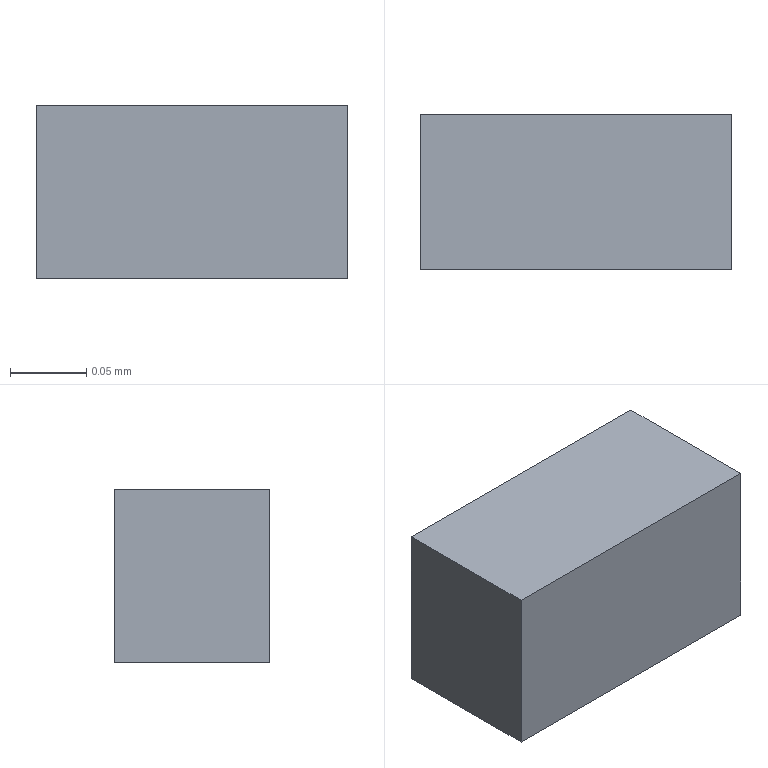Part | Creo | 1 solid | 6 faces | box 0.2032 x 0.1016 x 0.1136 mm | volume 0.002345 mm3 | plane 6
STEP:
#1=CARTESIAN_POINT('',(0.,0.,0.));
#2=DIRECTION('',(0.,0.,1.));
#3=DIRECTION('',(1.,0.,0.));
#4=AXIS2_PLACEMENT_3D('',#1,#2,#3);
#5=CARTESIAN_POINT('',(-0.1016,-0.0508,0.));
#6=VERTEX_POINT('',#5);
#7=CARTESIAN_POINT('',(0.1016,-0.0508,0.));
#8=VERTEX_POINT('',#7);
#9=CARTESIAN_POINT('',(-0.1016,-0.0508,0.));
#10=DIRECTION('',(1.,0.,0.));
#11=VECTOR('',#10,0.2032);
#12=LINE('',#9,#11);
#13=EDGE_CURVE('',#6,#8,#12,.T.);
#14=ORIENTED_EDGE('',*,*,#13,.T.);
#15=CARTESIAN_POINT('',(0.1016,0.0508,0.));
#16=VERTEX_POINT('',#15);
#17=CARTESIAN_POINT('',(0.1016,-0.0508,0.));
#18=DIRECTION('',(0.,1.,0.));
#19=VECTOR('',#18,0.1016);
#20=LINE('',#17,#19);
#21=EDGE_CURVE('',#8,#16,#20,.T.);
#22=ORIENTED_EDGE('',*,*,#21,.T.);
#23=CARTESIAN_POINT('',(-0.1016,0.0508,0.));
#24=VERTEX_POINT('',#23);
#25=CARTESIAN_POINT('',(0.1016,0.0508,0.));
#26=DIRECTION('',(-1.,0.,0.));
#27=VECTOR('',#26,0.2032);
#28=LINE('',#25,#27);
#29=EDGE_CURVE('',#16,#24,#28,.T.);
#30=ORIENTED_EDGE('',*,*,#29,.T.);
#31=CARTESIAN_POINT('',(-0.1016,0.0508,0.));
#32=DIRECTION('',(0.,-1.,0.));
#33=VECTOR('',#32,0.1016);
#34=LINE('',#31,#33);
#35=EDGE_CURVE('',#24,#6,#34,.T.);
#36=ORIENTED_EDGE('',*,*,#35,.T.);
#37=EDGE_LOOP('',(#14,#22,#30,#36));
#38=FACE_OUTER_BOUND('',#37,.F.);
#39=CARTESIAN_POINT('',(0.,0.,0.));
#40=DIRECTION('',(0.,0.,1.));
#41=DIRECTION('',(1.,0.,0.));
#42=AXIS2_PLACEMENT_3D('',#39,#40,#41);
#43=PLANE('',#42);
#44=ADVANCED_FACE('',(#38),#43,.F.);
#45=ORIENTED_EDGE('',*,*,#13,.F.);
#46=CARTESIAN_POINT('',(-0.1016,-0.0508,0.1136));
#47=VERTEX_POINT('',#46);
#48=CARTESIAN_POINT('',(-0.1016,-0.0508,0.));
#49=DIRECTION('',(0.,0.,1.));
#50=VECTOR('',#49,0.1136);
#51=LINE('',#48,#50);
#52=EDGE_CURVE('',#6,#47,#51,.T.);
#53=ORIENTED_EDGE('',*,*,#52,.T.);
#54=CARTESIAN_POINT('',(0.1016,-0.0508,0.1136));
#55=VERTEX_POINT('',#54);
#56=CARTESIAN_POINT('',(-0.1016,-0.0508,0.1136));
#57=DIRECTION('',(1.,0.,0.));
#58=VECTOR('',#57,0.2032);
#59=LINE('',#56,#58);
#60=EDGE_CURVE('',#47,#55,#59,.T.);
#61=ORIENTED_EDGE('',*,*,#60,.T.);
#62=CARTESIAN_POINT('',(0.1016,-0.0508,0.));
#63=DIRECTION('',(0.,0.,1.));
#64=VECTOR('',#63,0.1136);
#65=LINE('',#62,#64);
#66=EDGE_CURVE('',#8,#55,#65,.T.);
#67=ORIENTED_EDGE('',*,*,#66,.F.);
#68=EDGE_LOOP('',(#45,#53,#61,#67));
#69=FACE_OUTER_BOUND('',#68,.F.);
#70=CARTESIAN_POINT('',(-0.1016,-0.0508,0.));
#71=DIRECTION('',(0.,-1.,0.));
#72=DIRECTION('',(1.,0.,0.));
#73=AXIS2_PLACEMENT_3D('',#70,#71,#72);
#74=PLANE('',#73);
#75=ADVANCED_FACE('',(#69),#74,.T.);
#76=ORIENTED_EDGE('',*,*,#35,.F.);
#77=CARTESIAN_POINT('',(-0.1016,0.0508,0.1136));
#78=VERTEX_POINT('',#77);
#79=CARTESIAN_POINT('',(-0.1016,0.0508,0.));
#80=DIRECTION('',(0.,0.,1.));
#81=VECTOR('',#80,0.1136);
#82=LINE('',#79,#81);
#83=EDGE_CURVE('',#24,#78,#82,.T.);
#84=ORIENTED_EDGE('',*,*,#83,.T.);
#85=CARTESIAN_POINT('',(-0.1016,0.0508,0.1136));
#86=DIRECTION('',(0.,-1.,0.));
#87=VECTOR('',#86,0.1016);
#88=LINE('',#85,#87);
#89=EDGE_CURVE('',#78,#47,#88,.T.);
#90=ORIENTED_EDGE('',*,*,#89,.T.);
#91=ORIENTED_EDGE('',*,*,#52,.F.);
#92=EDGE_LOOP('',(#76,#84,#90,#91));
#93=FACE_OUTER_BOUND('',#92,.F.);
#94=CARTESIAN_POINT('',(-0.1016,0.0508,0.));
#95=DIRECTION('',(-1.,0.,0.));
#96=DIRECTION('',(0.,-1.,0.));
#97=AXIS2_PLACEMENT_3D('',#94,#95,#96);
#98=PLANE('',#97);
#99=ADVANCED_FACE('',(#93),#98,.T.);
#100=ORIENTED_EDGE('',*,*,#29,.F.);
#101=CARTESIAN_POINT('',(0.1016,0.0508,0.1136));
#102=VERTEX_POINT('',#101);
#103=CARTESIAN_POINT('',(0.1016,0.0508,0.));
#104=DIRECTION('',(0.,0.,1.));
#105=VECTOR('',#104,0.1136);
#106=LINE('',#103,#105);
#107=EDGE_CURVE('',#16,#102,#106,.T.);
#108=ORIENTED_EDGE('',*,*,#107,.T.);
#109=CARTESIAN_POINT('',(0.1016,0.0508,0.1136));
#110=DIRECTION('',(-1.,0.,0.));
#111=VECTOR('',#110,0.2032);
#112=LINE('',#109,#111);
#113=EDGE_CURVE('',#102,#78,#112,.T.);
#114=ORIENTED_EDGE('',*,*,#113,.T.);
#115=ORIENTED_EDGE('',*,*,#83,.F.);
#116=EDGE_LOOP('',(#100,#108,#114,#115));
#117=FACE_OUTER_BOUND('',#116,.F.);
#118=CARTESIAN_POINT('',(0.1016,0.0508,0.));
#119=DIRECTION('',(0.,1.,0.));
#120=DIRECTION('',(-1.,0.,0.));
#121=AXIS2_PLACEMENT_3D('',#118,#119,#120);
#122=PLANE('',#121);
#123=ADVANCED_FACE('',(#117),#122,.T.);
#124=ORIENTED_EDGE('',*,*,#21,.F.);
#125=ORIENTED_EDGE('',*,*,#66,.T.);
#126=CARTESIAN_POINT('',(0.1016,-0.0508,0.1136));
#127=DIRECTION('',(0.,1.,0.));
#128=VECTOR('',#127,0.1016);
#129=LINE('',#126,#128);
#130=EDGE_CURVE('',#55,#102,#129,.T.);
#131=ORIENTED_EDGE('',*,*,#130,.T.);
#132=ORIENTED_EDGE('',*,*,#107,.F.);
#133=EDGE_LOOP('',(#124,#125,#131,#132));
#134=FACE_OUTER_BOUND('',#133,.F.);
#135=CARTESIAN_POINT('',(0.1016,-0.0508,0.));
#136=DIRECTION('',(1.,0.,0.));
#137=DIRECTION('',(0.,1.,0.));
#138=AXIS2_PLACEMENT_3D('',#135,#136,#137);
#139=PLANE('',#138);
#140=ADVANCED_FACE('',(#134),#139,.T.);
#141=ORIENTED_EDGE('',*,*,#60,.F.);
#142=ORIENTED_EDGE('',*,*,#89,.F.);
#143=ORIENTED_EDGE('',*,*,#113,.F.);
#144=ORIENTED_EDGE('',*,*,#130,.F.);
#145=EDGE_LOOP('',(#141,#142,#143,#144));
#146=FACE_OUTER_BOUND('',#145,.F.);
#147=CARTESIAN_POINT('',(0.,0.,0.1136));
#148=DIRECTION('',(0.,0.,1.));
#149=DIRECTION('',(1.,0.,0.));
#150=AXIS2_PLACEMENT_3D('',#147,#148,#149);
#151=PLANE('',#150);
#152=ADVANCED_FACE('',(#146),#151,.T.);
#153=CLOSED_SHELL('',(#44,#75,#99,#123,#140,#152));
#154=MANIFOLD_SOLID_BREP('',#153);
#155=(LENGTH_UNIT()NAMED_UNIT(*)SI_UNIT(.MILLI.,.METRE.));
#156=UNCERTAINTY_MEASURE_WITH_UNIT(LENGTH_MEASURE(0.0000254),#155,'','');
#157=(NAMED_UNIT(*)PLANE_ANGLE_UNIT()SI_UNIT($,.RADIAN.));
#158=PLANE_ANGLE_MEASURE_WITH_UNIT(PLANE_ANGLE_MEASURE(0.01745),#157);
#159=(CONVERSION_BASED_UNIT('DEGREE',#158)NAMED_UNIT(*)PLANE_ANGLE_UNIT());
#160=(NAMED_UNIT(*)SI_UNIT($,.STERADIAN.)SOLID_ANGLE_UNIT());
#161=(GEOMETRIC_REPRESENTATION_CONTEXT(3)GLOBAL_UNCERTAINTY_ASSIGNED_CONTEXT((#156))GLOBAL_UNIT_ASSIGNED_CONTEXT((#155,#159,#160))REPRESENTATION_CONTEXT('',''));
#162=ADVANCED_BREP_SHAPE_REPRESENTATION('',(#4,#154),#161);